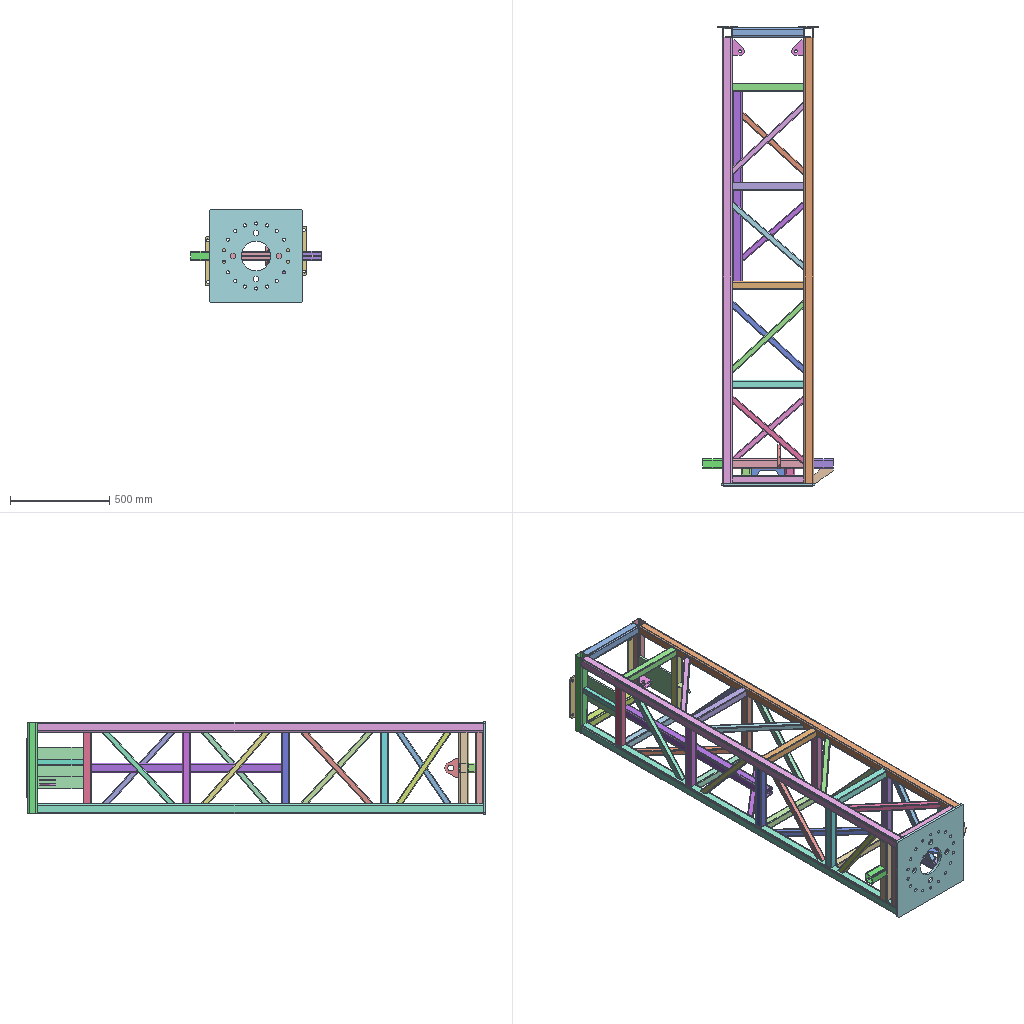Assembly | SolidWorks | 11 different items | 17 placed | box 660 x 2320 x 470 mm
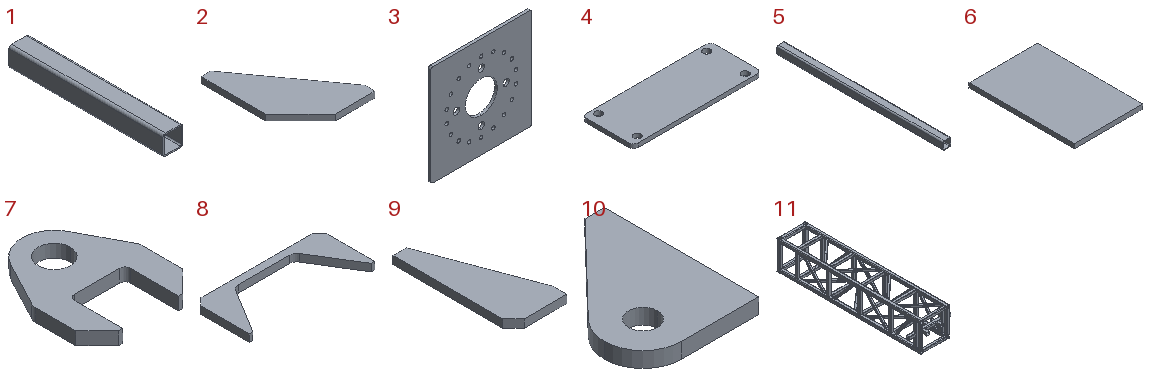Parts list (item | quantity | size | volume | features):
1 | x2 | 30 x 230 x 30 mm | 49151 mm3 | features WeldMemberFeat 1, WeldmentFeature 1
2 | x1 | 75 x 100 x 6 mm | 23775 mm3 | features Chamfer 1, Extrusion 1
3 | x1 | 470 x 12 x 470 mm | 2360354 mm3 | features HoleWzd 2, Extrusion 1
4 | x2 | 250 x 100 x 8 mm | 194387 mm3 | features Chamfer 1, Extrusion 1, Fillet 1, HoleWzd 1
5 | x1 | 50 x 1020 x 50 mm | 708692 mm3 | features WeldMemberFeat 1, WeldmentFeature 1
6 | x2 | 150 x 230 x 10 mm | 345000 mm3 | features Extrusion 1
7 | x1 | 100 x 120 x 12 mm | 75307 mm3 | features Extrusion 1
8 | x1 | 170 x 75 x 10 mm | 48537 mm3 | features Chamfer 1, Extrusion 1
9 | x1 | 40 x 90 x 6 mm | 14208 mm3 | features Chamfer 1, Extrusion 1
10 | x4 | 60 x 80 x 8 mm | 25848 mm3 | features Extrusion 1
11 | x1 | 660 x 2300 x 460 mm | 12314048 mm3 | features WeldCornerFeat 8, WeldMemberFeat 7, LPattern 3, CirPattern 2, 3DProfileFeature 1, MirrorSolid 1, RefAxis 1, WeldmentFeature 1
Mates (type | each side: item.copy, entity, surface, feature):
Coincident | 11.1 face plane Trim/Extend1 | 3.1 face plane Boss-Extrude1
Width | 3.1 face plane Boss-Extrude1 | 3.1 face plane Boss-Extrude1 | 11.1 face plane 50×50×4 - Missing(1) | 11.1 face plane 50×50×4 - Missing(1) | 2 times
Coincident | 11.1 face plane CirPattern1 | 2.1 face plane Boss-Extrude1
Coincident | 2.1 plane | assembly plane
Coordinate | 11.1 select_type:25 | assembly select_type:11
Coincident | 11.1 face plane Gb/t 6728—2002 square hollow section 50×50×4(3) | 2.1 face plane Boss-Extrude1
DistanceDim | 7.1 face plane Boss-Extrude1 | 11.1 face plane Gb/t 6728—2002 square hollow section 50×50×4(3)
Coincident | 11.1 face plane Gb/t 6728—2002 square hollow section 50×50×4(3) | 7.1 face plane Boss-Extrude1
Coincident | 6.1 face plane Boss-Extrude1 | 1.1 face plane Gb/t 6728—2002 square hollow section 30×30×2(1) | 2 times
Coincident | 6.1 face plane Boss-Extrude1 | 10.1 face plane Boss-Extrude1
Coincident | 10.1 face plane Boss-Extrude1 | 10.2 face plane Boss-Extrude1
Coincident | 6.1 face plane Boss-Extrude1 | 10.2 face plane Boss-Extrude1
DistanceDim | 10.2 face plane Boss-Extrude1 | 10.1 face plane Boss-Extrude1
Coincident | 11.1 face plane Gb/t 6728—2002 square hollow section 50×50×4(2) | 6.1 face plane Boss-Extrude1 | 2 times
Width | 6.1 face plane Boss-Extrude1 | 6.1 face plane Boss-Extrude1 | 1.1 face plane Gb/t 6728—2002 square hollow section 30×30×2(1) | 1.1 face plane Gb/t 6728—2002 square hollow section 30×30×2(1)
DistanceDim | 10.1 face plane Boss-Extrude1 | 6.1 face plane Boss-Extrude1
Coincident | 6.2 face plane Boss-Extrude1 | 1.2 face plane Gb/t 6728—2002 square hollow section 30×30×2(1) | 2 times
Coincident | 6.2 face plane Boss-Extrude1 | 10.3 face plane Boss-Extrude1
Coincident | 6.2 face plane Boss-Extrude1 | 10.4 face plane Boss-Extrude1
Coincident | 10.3 face plane Boss-Extrude1 | 10.4 face plane Boss-Extrude1
DistanceDim | 10.4 face plane Boss-Extrude1 | 6.2 face plane Boss-Extrude1
Width | 6.2 face plane Boss-Extrude1 | 6.2 face plane Boss-Extrude1 | 1.2 face plane Gb/t 6728—2002 square hollow section 30×30×2(1) | 1.2 face plane Gb/t 6728—2002 square hollow section 30×30×2(1)
DistanceDim | 10.3 face plane Boss-Extrude1 | 10.4 face plane Boss-Extrude1
Coincident | 11.1 face plane Gb/t 6728—2002 square hollow section 50×50×4(2) | 6.2 face plane Boss-Extrude1 | 2 times
Coincident | 11.1 face plane Gb/t 6728—2002 square hollow section 50×50×4(2) | 4.1 face plane Boss-Extrude1
DistanceDim | assembly plane | 4.1 face plane Boss-Extrude1
DistanceDim | 11.1 face plane Gb/t 6728—2002 square hollow section 50×50×4(2) | 4.1 face plane Boss-Extrude1
Coincident | 4.1 face plane Boss-Extrude1 | 4.2 face plane Boss-Extrude1
DistanceDim | 11.1 face plane Gb/t 6728—2002 square hollow section 50×50×4(2) | 4.2 face plane Boss-Extrude1
DistanceDim | assembly plane | 4.2 face plane Boss-Extrude1
Coincident | 11.1 face plane CirPattern1 | 5.1 face plane Gb/t 6728—2002 square hollow section 50×50×4(1)
DistanceDim | 5.1 face plane Gb/t 6728—2002 square hollow section 50×50×4(1) | 11.1 face plane CirPattern1
Coincident | 5.1 plane | assembly plane
Coincident | 11.1 face plane CirPattern1 | 9.1 face plane Boss-Extrude1
Coincident | 9.1 plane | assembly plane
DistanceDim | 6.1 face plane Boss-Extrude1 | 11.1 face plane 50×50×4 - Missing(1)
Coincident | 3.1 face plane Boss-Extrude1 | 8.1 face plane Boss-Extrude1
Coincident | 8.1 plane | assembly plane | 2 times
DistanceDim | 6.2 face plane Boss-Extrude1 | 11.1 face plane 50×50×4 - Missing(1)